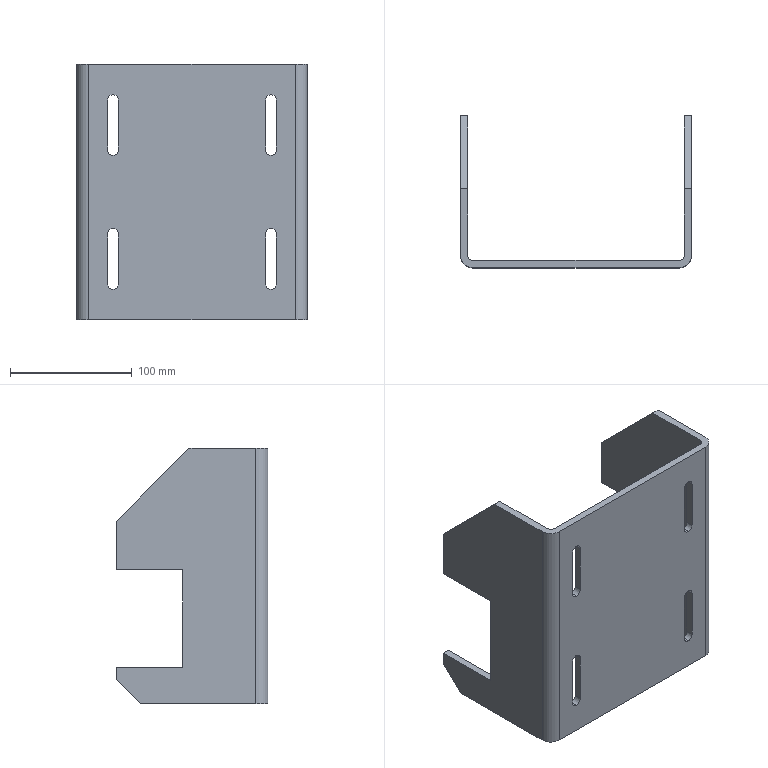Part | SolidWorks | features Chamfer 2, ICE 2, Extrusion 1 | 1 solid | 46 faces | box 190 x 125 x 210 mm | volume 444526 mm3 | plane 30 | cylinder 16 | commonest cylinder face diameters 9 x12 8 x2 20 x2
STEP:
#1=CARTESIAN_POINT('',(160.,-119.,135.));
#2=VERTEX_POINT('',#1);
#3=CARTESIAN_POINT('',(164.5,-119.,139.5));
#4=VERTEX_POINT('',#3);
#5=CARTESIAN_POINT('',(160.,-119.,139.5));
#6=DIRECTION('',(0.,-1.,0.));
#7=DIRECTION('',(0.,0.,-1.));
#8=AXIS2_PLACEMENT_3D('',#5,#6,#7);
#9=CIRCLE('',#8,4.5);
#10=EDGE_CURVE('',#2,#4,#9,.T.);
#11=ORIENTED_EDGE('',*,*,#10,.F.);
#12=CARTESIAN_POINT('',(160.,-125.,135.));
#13=VERTEX_POINT('',#12);
#14=CARTESIAN_POINT('',(160.,292.,135.));
#15=DIRECTION('',(0.,-1.,0.));
#16=VECTOR('',#15,1000.);
#17=LINE('',#14,#16);
#18=EDGE_CURVE('',#2,#13,#17,.T.);
#19=ORIENTED_EDGE('',*,*,#18,.T.);
#20=CARTESIAN_POINT('',(164.5,-125.,139.5));
#21=VERTEX_POINT('',#20);
#22=CARTESIAN_POINT('',(160.,-125.,139.5));
#23=DIRECTION('',(0.,-1.,0.));
#24=DIRECTION('',(0.,0.,-1.));
#25=AXIS2_PLACEMENT_3D('',#22,#23,#24);
#26=CIRCLE('',#25,4.5);
#27=EDGE_CURVE('',#13,#21,#26,.T.);
#28=ORIENTED_EDGE('',*,*,#27,.T.);
#29=CARTESIAN_POINT('',(164.5,292.,139.5));
#30=DIRECTION('',(0.,-1.,0.));
#31=VECTOR('',#30,1000.);
#32=LINE('',#29,#31);
#33=EDGE_CURVE('',#4,#21,#32,.T.);
#34=ORIENTED_EDGE('',*,*,#33,.F.);
#35=EDGE_LOOP('',(#11,#19,#28,#34));
#36=FACE_OUTER_BOUND('',#35,.T.);
#37=CARTESIAN_POINT('',(160.,292.,139.5));
#38=DIRECTION('',(0.,-1.,0.));
#39=DIRECTION('',(0.,0.,-1.));
#40=AXIS2_PLACEMENT_3D('',#37,#38,#39);
#41=CYLINDRICAL_SURFACE('',#40,4.5);
#42=ADVANCED_FACE('',(#36),#41,.F.);
#43=CARTESIAN_POINT('',(30.,-119.,25.));
#44=VERTEX_POINT('',#43);
#45=CARTESIAN_POINT('',(34.5,-119.,29.5));
#46=VERTEX_POINT('',#45);
#47=CARTESIAN_POINT('',(30.,-119.,29.5));
#48=DIRECTION('',(0.,-1.,0.));
#49=DIRECTION('',(0.,0.,-1.));
#50=AXIS2_PLACEMENT_3D('',#47,#48,#49);
#51=CIRCLE('',#50,4.5);
#52=EDGE_CURVE('',#44,#46,#51,.T.);
#53=ORIENTED_EDGE('',*,*,#52,.F.);
#54=CARTESIAN_POINT('',(30.,-125.,25.));
#55=VERTEX_POINT('',#54);
#56=CARTESIAN_POINT('',(30.,292.,25.));
#57=DIRECTION('',(0.,-1.,0.));
#58=VECTOR('',#57,1000.);
#59=LINE('',#56,#58);
#60=EDGE_CURVE('',#44,#55,#59,.T.);
#61=ORIENTED_EDGE('',*,*,#60,.T.);
#62=CARTESIAN_POINT('',(34.5,-125.,29.5));
#63=VERTEX_POINT('',#62);
#64=CARTESIAN_POINT('',(30.,-125.,29.5));
#65=DIRECTION('',(0.,-1.,0.));
#66=DIRECTION('',(0.,0.,-1.));
#67=AXIS2_PLACEMENT_3D('',#64,#65,#66);
#68=CIRCLE('',#67,4.5);
#69=EDGE_CURVE('',#55,#63,#68,.T.);
#70=ORIENTED_EDGE('',*,*,#69,.T.);
#71=CARTESIAN_POINT('',(34.5,292.,29.5));
#72=DIRECTION('',(0.,-1.,0.));
#73=VECTOR('',#72,1000.);
#74=LINE('',#71,#73);
#75=EDGE_CURVE('',#46,#63,#74,.T.);
#76=ORIENTED_EDGE('',*,*,#75,.F.);
#77=EDGE_LOOP('',(#53,#61,#70,#76));
#78=FACE_OUTER_BOUND('',#77,.T.);
#79=CARTESIAN_POINT('',(30.,292.,29.5));
#80=DIRECTION('',(0.,-1.,0.));
#81=DIRECTION('',(0.,0.,-1.));
#82=AXIS2_PLACEMENT_3D('',#79,#80,#81);
#83=CYLINDRICAL_SURFACE('',#82,4.5);
#84=ADVANCED_FACE('',(#78),#83,.F.);
#85=CARTESIAN_POINT('',(160.,-119.,25.));
#86=VERTEX_POINT('',#85);
#87=CARTESIAN_POINT('',(164.5,-119.,29.5));
#88=VERTEX_POINT('',#87);
#89=CARTESIAN_POINT('',(160.,-119.,29.5));
#90=DIRECTION('',(0.,-1.,0.));
#91=DIRECTION('',(0.,0.,-1.));
#92=AXIS2_PLACEMENT_3D('',#89,#90,#91);
#93=CIRCLE('',#92,4.5);
#94=EDGE_CURVE('',#86,#88,#93,.T.);
#95=ORIENTED_EDGE('',*,*,#94,.F.);
#96=CARTESIAN_POINT('',(160.,-125.,25.));
#97=VERTEX_POINT('',#96);
#98=CARTESIAN_POINT('',(160.,292.,25.));
#99=DIRECTION('',(0.,-1.,0.));
#100=VECTOR('',#99,1000.);
#101=LINE('',#98,#100);
#102=EDGE_CURVE('',#86,#97,#101,.T.);
#103=ORIENTED_EDGE('',*,*,#102,.T.);
#104=CARTESIAN_POINT('',(164.5,-125.,29.5));
#105=VERTEX_POINT('',#104);
#106=CARTESIAN_POINT('',(160.,-125.,29.5));
#107=DIRECTION('',(0.,-1.,0.));
#108=DIRECTION('',(0.,0.,-1.));
#109=AXIS2_PLACEMENT_3D('',#106,#107,#108);
#110=CIRCLE('',#109,4.5);
#111=EDGE_CURVE('',#97,#105,#110,.T.);
#112=ORIENTED_EDGE('',*,*,#111,.T.);
#113=CARTESIAN_POINT('',(164.5,292.,29.5));
#114=DIRECTION('',(0.,-1.,0.));
#115=VECTOR('',#114,1000.);
#116=LINE('',#113,#115);
#117=EDGE_CURVE('',#88,#105,#116,.T.);
#118=ORIENTED_EDGE('',*,*,#117,.F.);
#119=EDGE_LOOP('',(#95,#103,#112,#118));
#120=FACE_OUTER_BOUND('',#119,.T.);
#121=CARTESIAN_POINT('',(160.,292.,29.5));
#122=DIRECTION('',(0.,-1.,0.));
#123=DIRECTION('',(0.,0.,-1.));
#124=AXIS2_PLACEMENT_3D('',#121,#122,#123);
#125=CYLINDRICAL_SURFACE('',#124,4.5);
#126=ADVANCED_FACE('',(#120),#125,.F.);
#127=CARTESIAN_POINT('',(30.,-119.,135.));
#128=VERTEX_POINT('',#127);
#129=CARTESIAN_POINT('',(34.5,-119.,139.5));
#130=VERTEX_POINT('',#129);
#131=CARTESIAN_POINT('',(30.,-119.,139.5));
#132=DIRECTION('',(0.,-1.,0.));
#133=DIRECTION('',(0.,0.,-1.));
#134=AXIS2_PLACEMENT_3D('',#131,#132,#133);
#135=CIRCLE('',#134,4.5);
#136=EDGE_CURVE('',#128,#130,#135,.T.);
#137=ORIENTED_EDGE('',*,*,#136,.F.);
#138=CARTESIAN_POINT('',(30.,-125.,135.));
#139=VERTEX_POINT('',#138);
#140=CARTESIAN_POINT('',(30.,292.,135.));
#141=DIRECTION('',(0.,-1.,0.));
#142=VECTOR('',#141,1000.);
#143=LINE('',#140,#142);
#144=EDGE_CURVE('',#128,#139,#143,.T.);
#145=ORIENTED_EDGE('',*,*,#144,.T.);
#146=CARTESIAN_POINT('',(34.5,-125.,139.5));
#147=VERTEX_POINT('',#146);
#148=CARTESIAN_POINT('',(30.,-125.,139.5));
#149=DIRECTION('',(0.,-1.,0.));
#150=DIRECTION('',(0.,0.,-1.));
#151=AXIS2_PLACEMENT_3D('',#148,#149,#150);
#152=CIRCLE('',#151,4.5);
#153=EDGE_CURVE('',#139,#147,#152,.T.);
#154=ORIENTED_EDGE('',*,*,#153,.T.);
#155=CARTESIAN_POINT('',(34.5,292.,139.5));
#156=DIRECTION('',(0.,-1.,0.));
#157=VECTOR('',#156,1000.);
#158=LINE('',#155,#157);
#159=EDGE_CURVE('',#130,#147,#158,.T.);
#160=ORIENTED_EDGE('',*,*,#159,.F.);
#161=EDGE_LOOP('',(#137,#145,#154,#160));
#162=FACE_OUTER_BOUND('',#161,.T.);
#163=CARTESIAN_POINT('',(30.,292.,139.5));
#164=DIRECTION('',(0.,-1.,0.));
#165=DIRECTION('',(0.,0.,-1.));
#166=AXIS2_PLACEMENT_3D('',#163,#164,#165);
#167=CYLINDRICAL_SURFACE('',#166,4.5);
#168=ADVANCED_FACE('',(#162),#167,.F.);
#169=CARTESIAN_POINT('',(6.,0.,150.));
#170=VERTEX_POINT('',#169);
#171=CARTESIAN_POINT('',(6.,0.,110.));
#172=VERTEX_POINT('',#171);
#173=CARTESIAN_POINT('',(6.,0.,210.));
#174=DIRECTION('',(0.,0.,-1.));
#175=VECTOR('',#174,1000.);
#176=LINE('',#173,#175);
#177=EDGE_CURVE('',#170,#172,#176,.T.);
#178=ORIENTED_EDGE('',*,*,#177,.T.);
#179=CARTESIAN_POINT('',(0.,0.,110.));
#180=VERTEX_POINT('',#179);
#181=CARTESIAN_POINT('',(6.,0.,110.));
#182=DIRECTION('',(-1.,0.,0.));
#183=VECTOR('',#182,1000.);
#184=LINE('',#181,#183);
#185=EDGE_CURVE('',#172,#180,#184,.T.);
#186=ORIENTED_EDGE('',*,*,#185,.T.);
#187=CARTESIAN_POINT('',(0.,0.,150.));
#188=VERTEX_POINT('',#187);
#189=CARTESIAN_POINT('',(0.,0.,210.));
#190=DIRECTION('',(0.,0.,-1.));
#191=VECTOR('',#190,1000.);
#192=LINE('',#189,#191);
#193=EDGE_CURVE('',#188,#180,#192,.T.);
#194=ORIENTED_EDGE('',*,*,#193,.F.);
#195=CARTESIAN_POINT('',(6.,0.,150.));
#196=DIRECTION('',(1.,0.,0.));
#197=VECTOR('',#196,1000.);
#198=LINE('',#195,#197);
#199=EDGE_CURVE('',#188,#170,#198,.T.);
#200=ORIENTED_EDGE('',*,*,#199,.T.);
#201=EDGE_LOOP('',(#178,#186,#194,#200));
#202=FACE_OUTER_BOUND('',#201,.T.);
#203=CARTESIAN_POINT('',(6.,0.,210.));
#204=DIRECTION('',(0.,-1.,0.));
#205=DIRECTION('',(0.,0.,-1.));
#206=AXIS2_PLACEMENT_3D('',#203,#204,#205);
#207=PLANE('',#206);
#208=ADVANCED_FACE('',(#202),#207,.F.);
#209=CARTESIAN_POINT('',(190.,0.,150.));
#210=VERTEX_POINT('',#209);
#211=CARTESIAN_POINT('',(190.,0.,110.));
#212=VERTEX_POINT('',#211);
#213=CARTESIAN_POINT('',(190.,0.,210.));
#214=DIRECTION('',(0.,0.,-1.));
#215=VECTOR('',#214,1000.);
#216=LINE('',#213,#215);
#217=EDGE_CURVE('',#210,#212,#216,.T.);
#218=ORIENTED_EDGE('',*,*,#217,.T.);
#219=CARTESIAN_POINT('',(184.,0.,110.));
#220=VERTEX_POINT('',#219);
#221=CARTESIAN_POINT('',(190.,0.,110.));
#222=DIRECTION('',(-1.,0.,0.));
#223=VECTOR('',#222,1000.);
#224=LINE('',#221,#223);
#225=EDGE_CURVE('',#212,#220,#224,.T.);
#226=ORIENTED_EDGE('',*,*,#225,.T.);
#227=CARTESIAN_POINT('',(184.,0.,150.));
#228=VERTEX_POINT('',#227);
#229=CARTESIAN_POINT('',(184.,0.,210.));
#230=DIRECTION('',(0.,0.,-1.));
#231=VECTOR('',#230,1000.);
#232=LINE('',#229,#231);
#233=EDGE_CURVE('',#228,#220,#232,.T.);
#234=ORIENTED_EDGE('',*,*,#233,.F.);
#235=CARTESIAN_POINT('',(190.,0.,150.));
#236=DIRECTION('',(1.,0.,0.));
#237=VECTOR('',#236,1000.);
#238=LINE('',#235,#237);
#239=EDGE_CURVE('',#228,#210,#238,.T.);
#240=ORIENTED_EDGE('',*,*,#239,.T.);
#241=EDGE_LOOP('',(#218,#226,#234,#240));
#242=FACE_OUTER_BOUND('',#241,.T.);
#243=CARTESIAN_POINT('',(190.,0.,210.));
#244=DIRECTION('',(0.,-1.,0.));
#245=DIRECTION('',(0.,0.,-1.));
#246=AXIS2_PLACEMENT_3D('',#243,#244,#245);
#247=PLANE('',#246);
#248=ADVANCED_FACE('',(#242),#247,.F.);
#249=CARTESIAN_POINT('',(0.,0.,30.));
#250=VERTEX_POINT('',#249);
#251=CARTESIAN_POINT('',(0.,0.,20.));
#252=VERTEX_POINT('',#251);
#253=CARTESIAN_POINT('',(0.,0.,210.));
#254=DIRECTION('',(0.,0.,-1.));
#255=VECTOR('',#254,1000.);
#256=LINE('',#253,#255);
#257=EDGE_CURVE('',#250,#252,#256,.T.);
#258=ORIENTED_EDGE('',*,*,#257,.F.);
#259=CARTESIAN_POINT('',(6.,0.,30.));
#260=VERTEX_POINT('',#259);
#261=CARTESIAN_POINT('',(6.,0.,30.));
#262=DIRECTION('',(1.,0.,0.));
#263=VECTOR('',#262,1000.);
#264=LINE('',#261,#263);
#265=EDGE_CURVE('',#250,#260,#264,.T.);
#266=ORIENTED_EDGE('',*,*,#265,.T.);
#267=CARTESIAN_POINT('',(6.,0.,20.));
#268=VERTEX_POINT('',#267);
#269=CARTESIAN_POINT('',(6.,0.,210.));
#270=DIRECTION('',(0.,0.,-1.));
#271=VECTOR('',#270,1000.);
#272=LINE('',#269,#271);
#273=EDGE_CURVE('',#260,#268,#272,.T.);
#274=ORIENTED_EDGE('',*,*,#273,.T.);
#275=CARTESIAN_POINT('',(6.,0.,20.));
#276=DIRECTION('',(-1.,0.,0.));
#277=VECTOR('',#276,1000.);
#278=LINE('',#275,#277);
#279=EDGE_CURVE('',#268,#252,#278,.T.);
#280=ORIENTED_EDGE('',*,*,#279,.T.);
#281=EDGE_LOOP('',(#258,#266,#274,#280));
#282=FACE_OUTER_BOUND('',#281,.T.);
#283=CARTESIAN_POINT('',(6.,0.,210.));
#284=DIRECTION('',(0.,-1.,0.));
#285=DIRECTION('',(0.,0.,-1.));
#286=AXIS2_PLACEMENT_3D('',#283,#284,#285);
#287=PLANE('',#286);
#288=ADVANCED_FACE('',(#282),#287,.F.);
#289=ORIENTED_EDGE('',*,*,#193,.T.);
#290=CARTESIAN_POINT('',(0.,-55.,110.));
#291=VERTEX_POINT('',#290);
#292=CARTESIAN_POINT('',(0.,0.,110.));
#293=DIRECTION('',(0.,-1.,0.));
#294=VECTOR('',#293,1000.);
#295=LINE('',#292,#294);
#296=EDGE_CURVE('',#180,#291,#295,.T.);
#297=ORIENTED_EDGE('',*,*,#296,.T.);
#298=CARTESIAN_POINT('',(0.,-55.,30.));
#299=VERTEX_POINT('',#298);
#300=CARTESIAN_POINT('',(0.,-55.,210.));
#301=DIRECTION('',(0.,0.,-1.));
#302=VECTOR('',#301,1000.);
#303=LINE('',#300,#302);
#304=EDGE_CURVE('',#291,#299,#303,.T.);
#305=ORIENTED_EDGE('',*,*,#304,.T.);
#306=CARTESIAN_POINT('',(0.,0.,30.));
#307=DIRECTION('',(0.,1.,0.));
#308=VECTOR('',#307,1000.);
#309=LINE('',#306,#308);
#310=EDGE_CURVE('',#299,#250,#309,.T.);
#311=ORIENTED_EDGE('',*,*,#310,.T.);
#312=ORIENTED_EDGE('',*,*,#257,.T.);
#313=CARTESIAN_POINT('',(0.,-20.,0.));
#314=VERTEX_POINT('',#313);
#315=CARTESIAN_POINT('',(0.,0.,20.));
#316=DIRECTION('',(0.,-0.7071,-0.7071));
#317=VECTOR('',#316,1000.);
#318=LINE('',#315,#317);
#319=EDGE_CURVE('',#252,#314,#318,.T.);
#320=ORIENTED_EDGE('',*,*,#319,.T.);
#321=CARTESIAN_POINT('',(0.,-115.,0.));
#322=VERTEX_POINT('',#321);
#323=CARTESIAN_POINT('',(0.,0.,0.));
#324=DIRECTION('',(0.,-1.,0.));
#325=VECTOR('',#324,1000.);
#326=LINE('',#323,#325);
#327=EDGE_CURVE('',#314,#322,#326,.T.);
#328=ORIENTED_EDGE('',*,*,#327,.T.);
#329=CARTESIAN_POINT('',(0.,-115.,210.));
#330=VERTEX_POINT('',#329);
#331=CARTESIAN_POINT('',(0.,-115.,210.));
#332=DIRECTION('',(0.,0.,-1.));
#333=VECTOR('',#332,1000.);
#334=LINE('',#331,#333);
#335=EDGE_CURVE('',#330,#322,#334,.T.);
#336=ORIENTED_EDGE('',*,*,#335,.F.);
#337=CARTESIAN_POINT('',(0.,-60.,210.));
#338=VERTEX_POINT('',#337);
#339=CARTESIAN_POINT('',(0.,0.,210.));
#340=DIRECTION('',(0.,-1.,0.));
#341=VECTOR('',#340,1000.);
#342=LINE('',#339,#341);
#343=EDGE_CURVE('',#338,#330,#342,.T.);
#344=ORIENTED_EDGE('',*,*,#343,.F.);
#345=CARTESIAN_POINT('',(0.,-60.,210.));
#346=DIRECTION('',(0.,0.7071,-0.7071));
#347=VECTOR('',#346,1000.);
#348=LINE('',#345,#347);
#349=EDGE_CURVE('',#338,#188,#348,.T.);
#350=ORIENTED_EDGE('',*,*,#349,.T.);
#351=EDGE_LOOP('',(#289,#297,#305,#311,#312,#320,#328,#336,#344,#350));
#352=FACE_OUTER_BOUND('',#351,.T.);
#353=CARTESIAN_POINT('',(0.,0.,210.));
#354=DIRECTION('',(1.,0.,0.));
#355=DIRECTION('',(0.,0.,-1.));
#356=AXIS2_PLACEMENT_3D('',#353,#354,#355);
#357=PLANE('',#356);
#358=ADVANCED_FACE('',(#352),#357,.F.);
#359=CARTESIAN_POINT('',(10.,-125.,0.));
#360=VERTEX_POINT('',#359);
#361=CARTESIAN_POINT('',(10.,-115.,0.));
#362=DIRECTION('',(0.,0.,1.));
#363=DIRECTION('',(1.,0.,0.));
#364=AXIS2_PLACEMENT_3D('',#361,#362,#363);
#365=CIRCLE('',#364,10.);
#366=EDGE_CURVE('',#322,#360,#365,.T.);
#367=ORIENTED_EDGE('',*,*,#366,.T.);
#368=CARTESIAN_POINT('',(10.,-125.,210.));
#369=VERTEX_POINT('',#368);
#370=CARTESIAN_POINT('',(10.,-125.,210.));
#371=DIRECTION('',(0.,0.,-1.));
#372=VECTOR('',#371,1000.);
#373=LINE('',#370,#372);
#374=EDGE_CURVE('',#369,#360,#373,.T.);
#375=ORIENTED_EDGE('',*,*,#374,.F.);
#376=CARTESIAN_POINT('',(10.,-115.,210.));
#377=DIRECTION('',(0.,0.,1.));
#378=DIRECTION('',(1.,0.,0.));
#379=AXIS2_PLACEMENT_3D('',#376,#377,#378);
#380=CIRCLE('',#379,10.);
#381=EDGE_CURVE('',#330,#369,#380,.T.);
#382=ORIENTED_EDGE('',*,*,#381,.F.);
#383=ORIENTED_EDGE('',*,*,#335,.T.);
#384=EDGE_LOOP('',(#367,#375,#382,#383));
#385=FACE_OUTER_BOUND('',#384,.T.);
#386=CARTESIAN_POINT('',(10.,-115.,210.));
#387=DIRECTION('',(0.,0.,-1.));
#388=DIRECTION('',(-1.,0.,0.));
#389=AXIS2_PLACEMENT_3D('',#386,#387,#388);
#390=CYLINDRICAL_SURFACE('',#389,10.);
#391=ADVANCED_FACE('',(#385),#390,.T.);
#392=CARTESIAN_POINT('',(155.5,-125.,180.5));
#393=VERTEX_POINT('',#392);
#394=CARTESIAN_POINT('',(155.5,-125.,139.5));
#395=VERTEX_POINT('',#394);
#396=CARTESIAN_POINT('',(155.5,-125.,180.5));
#397=DIRECTION('',(0.,0.,-1.));
#398=VECTOR('',#397,1000.);
#399=LINE('',#396,#398);
#400=EDGE_CURVE('',#393,#395,#399,.T.);
#401=ORIENTED_EDGE('',*,*,#400,.F.);
#402=CARTESIAN_POINT('',(164.5,-125.,180.5));
#403=VERTEX_POINT('',#402);
#404=CARTESIAN_POINT('',(160.,-125.,180.5));
#405=DIRECTION('',(0.,-1.,0.));
#406=DIRECTION('',(0.,0.,-1.));
#407=AXIS2_PLACEMENT_3D('',#404,#405,#406);
#408=CIRCLE('',#407,4.5);
#409=EDGE_CURVE('',#403,#393,#408,.T.);
#410=ORIENTED_EDGE('',*,*,#409,.F.);
#411=CARTESIAN_POINT('',(164.5,-125.,180.5));
#412=DIRECTION('',(0.,0.,1.));
#413=VECTOR('',#412,1000.);
#414=LINE('',#411,#413);
#415=EDGE_CURVE('',#21,#403,#414,.T.);
#416=ORIENTED_EDGE('',*,*,#415,.F.);
#417=ORIENTED_EDGE('',*,*,#27,.F.);
#418=CARTESIAN_POINT('',(160.,-125.,139.5));
#419=DIRECTION('',(0.,-1.,0.));
#420=DIRECTION('',(0.,0.,-1.));
#421=AXIS2_PLACEMENT_3D('',#418,#419,#420);
#422=CIRCLE('',#421,4.5);
#423=EDGE_CURVE('',#395,#13,#422,.T.);
#424=ORIENTED_EDGE('',*,*,#423,.F.);
#425=EDGE_LOOP('',(#401,#410,#416,#417,#424));
#426=FACE_BOUND('',#425,.T.);
#427=CARTESIAN_POINT('',(25.5,-125.,70.5));
#428=VERTEX_POINT('',#427);
#429=CARTESIAN_POINT('',(25.5,-125.,29.5));
#430=VERTEX_POINT('',#429);
#431=CARTESIAN_POINT('',(25.5,-125.,70.5));
#432=DIRECTION('',(0.,0.,-1.));
#433=VECTOR('',#432,1000.);
#434=LINE('',#431,#433);
#435=EDGE_CURVE('',#428,#430,#434,.T.);
#436=ORIENTED_EDGE('',*,*,#435,.F.);
#437=CARTESIAN_POINT('',(34.5,-125.,70.5));
#438=VERTEX_POINT('',#437);
#439=CARTESIAN_POINT('',(30.,-125.,70.5));
#440=DIRECTION('',(0.,-1.,0.));
#441=DIRECTION('',(0.,0.,-1.));
#442=AXIS2_PLACEMENT_3D('',#439,#440,#441);
#443=CIRCLE('',#442,4.5);
#444=EDGE_CURVE('',#438,#428,#443,.T.);
#445=ORIENTED_EDGE('',*,*,#444,.F.);
#446=CARTESIAN_POINT('',(34.5,-125.,70.5));
#447=DIRECTION('',(0.,0.,1.));
#448=VECTOR('',#447,1000.);
#449=LINE('',#446,#448);
#450=EDGE_CURVE('',#63,#438,#449,.T.);
#451=ORIENTED_EDGE('',*,*,#450,.F.);
#452=ORIENTED_EDGE('',*,*,#69,.F.);
#453=CARTESIAN_POINT('',(30.,-125.,29.5));
#454=DIRECTION('',(0.,-1.,0.));
#455=DIRECTION('',(0.,0.,-1.));
#456=AXIS2_PLACEMENT_3D('',#453,#454,#455);
#457=CIRCLE('',#456,4.5);
#458=EDGE_CURVE('',#430,#55,#457,.T.);
#459=ORIENTED_EDGE('',*,*,#458,.F.);
#460=EDGE_LOOP('',(#436,#445,#451,#452,#459));
#461=FACE_BOUND('',#460,.T.);
#462=CARTESIAN_POINT('',(155.5,-125.,70.5));
#463=VERTEX_POINT('',#462);
#464=CARTESIAN_POINT('',(155.5,-125.,29.5));
#465=VERTEX_POINT('',#464);
#466=CARTESIAN_POINT('',(155.5,-125.,70.5));
#467=DIRECTION('',(0.,0.,-1.));
#468=VECTOR('',#467,1000.);
#469=LINE('',#466,#468);
#470=EDGE_CURVE('',#463,#465,#469,.T.);
#471=ORIENTED_EDGE('',*,*,#470,.F.);
#472=CARTESIAN_POINT('',(164.5,-125.,70.5));
#473=VERTEX_POINT('',#472);
#474=CARTESIAN_POINT('',(160.,-125.,70.5));
#475=DIRECTION('',(0.,-1.,0.));
#476=DIRECTION('',(0.,0.,-1.));
#477=AXIS2_PLACEMENT_3D('',#474,#475,#476);
#478=CIRCLE('',#477,4.5);
#479=EDGE_CURVE('',#473,#463,#478,.T.);
#480=ORIENTED_EDGE('',*,*,#479,.F.);
#481=CARTESIAN_POINT('',(164.5,-125.,70.5));
#482=DIRECTION('',(0.,0.,1.));
#483=VECTOR('',#482,1000.);
#484=LINE('',#481,#483);
#485=EDGE_CURVE('',#105,#473,#484,.T.);
#486=ORIENTED_EDGE('',*,*,#485,.F.);
#487=ORIENTED_EDGE('',*,*,#111,.F.);
#488=CARTESIAN_POINT('',(160.,-125.,29.5));
#489=DIRECTION('',(0.,-1.,0.));
#490=DIRECTION('',(0.,0.,-1.));
#491=AXIS2_PLACEMENT_3D('',#488,#489,#490);
#492=CIRCLE('',#491,4.5);
#493=EDGE_CURVE('',#465,#97,#492,.T.);
#494=ORIENTED_EDGE('',*,*,#493,.F.);
#495=EDGE_LOOP('',(#471,#480,#486,#487,#494));
#496=FACE_BOUND('',#495,.T.);
#497=CARTESIAN_POINT('',(25.5,-125.,180.5));
#498=VERTEX_POINT('',#497);
#499=CARTESIAN_POINT('',(25.5,-125.,139.5));
#500=VERTEX_POINT('',#499);
#501=CARTESIAN_POINT('',(25.5,-125.,180.5));
#502=DIRECTION('',(0.,0.,-1.));
#503=VECTOR('',#502,1000.);
#504=LINE('',#501,#503);
#505=EDGE_CURVE('',#498,#500,#504,.T.);
#506=ORIENTED_EDGE('',*,*,#505,.F.);
#507=CARTESIAN_POINT('',(34.5,-125.,180.5));
#508=VERTEX_POINT('',#507);
#509=CARTESIAN_POINT('',(30.,-125.,180.5));
#510=DIRECTION('',(0.,-1.,0.));
#511=DIRECTION('',(0.,0.,-1.));
#512=AXIS2_PLACEMENT_3D('',#509,#510,#511);
#513=CIRCLE('',#512,4.5);
#514=EDGE_CURVE('',#508,#498,#513,.T.);
#515=ORIENTED_EDGE('',*,*,#514,.F.);
#516=CARTESIAN_POINT('',(34.5,-125.,180.5));
#517=DIRECTION('',(0.,0.,1.));
#518=VECTOR('',#517,1000.);
#519=LINE('',#516,#518);
#520=EDGE_CURVE('',#147,#508,#519,.T.);
#521=ORIENTED_EDGE('',*,*,#520,.F.);
#522=ORIENTED_EDGE('',*,*,#153,.F.);
#523=CARTESIAN_POINT('',(30.,-125.,139.5));
#524=DIRECTION('',(0.,-1.,0.));
#525=DIRECTION('',(0.,0.,-1.));
#526=AXIS2_PLACEMENT_3D('',#523,#524,#525);
#527=CIRCLE('',#526,4.5);
#528=EDGE_CURVE('',#500,#139,#527,.T.);
#529=ORIENTED_EDGE('',*,*,#528,.F.);
#530=EDGE_LOOP('',(#506,#515,#521,#522,#529));
#531=FACE_BOUND('',#530,.T.);
#532=CARTESIAN_POINT('',(180.,-125.,0.));
#533=VERTEX_POINT('',#532);
#534=CARTESIAN_POINT('',(10.,-125.,0.));
#535=DIRECTION('',(1.,0.,0.));
#536=VECTOR('',#535,1000.);
#537=LINE('',#534,#536);
#538=EDGE_CURVE('',#360,#533,#537,.T.);
#539=ORIENTED_EDGE('',*,*,#538,.T.);
#540=CARTESIAN_POINT('',(180.,-125.,210.));
#541=VERTEX_POINT('',#540);
#542=CARTESIAN_POINT('',(180.,-125.,210.));
#543=DIRECTION('',(0.,0.,-1.));
#544=VECTOR('',#543,1000.);
#545=LINE('',#542,#544);
#546=EDGE_CURVE('',#541,#533,#545,.T.);
#547=ORIENTED_EDGE('',*,*,#546,.F.);
#548=CARTESIAN_POINT('',(10.,-125.,210.));
#549=DIRECTION('',(1.,0.,0.));
#550=VECTOR('',#549,1000.);
#551=LINE('',#548,#550);
#552=EDGE_CURVE('',#369,#541,#551,.T.);
#553=ORIENTED_EDGE('',*,*,#552,.F.);
#554=ORIENTED_EDGE('',*,*,#374,.T.);
#555=EDGE_LOOP('',(#539,#547,#553,#554));
#556=FACE_OUTER_BOUND('',#555,.T.);
#557=CARTESIAN_POINT('',(10.,-125.,210.));
#558=DIRECTION('',(0.,1.,0.));
#559=DIRECTION('',(0.,0.,1.));
#560=AXIS2_PLACEMENT_3D('',#557,#558,#559);
#561=PLANE('',#560);
#562=ADVANCED_FACE('',(#426,#461,#496,#531,#556),#561,.F.);
#563=CARTESIAN_POINT('',(190.,-115.,0.));
#564=VERTEX_POINT('',#563);
#565=CARTESIAN_POINT('',(180.,-115.,0.));
#566=DIRECTION('',(0.,0.,1.));
#567=DIRECTION('',(1.,0.,0.));
#568=AXIS2_PLACEMENT_3D('',#565,#566,#567);
#569=CIRCLE('',#568,10.);
#570=EDGE_CURVE('',#533,#564,#569,.T.);
#571=ORIENTED_EDGE('',*,*,#570,.T.);
#572=CARTESIAN_POINT('',(190.,-115.,210.));
#573=VERTEX_POINT('',#572);
#574=CARTESIAN_POINT('',(190.,-115.,210.));
#575=DIRECTION('',(0.,0.,-1.));
#576=VECTOR('',#575,1000.);
#577=LINE('',#574,#576);
#578=EDGE_CURVE('',#573,#564,#577,.T.);
#579=ORIENTED_EDGE('',*,*,#578,.F.);
#580=CARTESIAN_POINT('',(180.,-115.,210.));
#581=DIRECTION('',(0.,0.,1.));
#582=DIRECTION('',(1.,0.,0.));
#583=AXIS2_PLACEMENT_3D('',#580,#581,#582);
#584=CIRCLE('',#583,10.);
#585=EDGE_CURVE('',#541,#573,#584,.T.);
#586=ORIENTED_EDGE('',*,*,#585,.F.);
#587=ORIENTED_EDGE('',*,*,#546,.T.);
#588=EDGE_LOOP('',(#571,#579,#586,#587));
#589=FACE_OUTER_BOUND('',#588,.T.);
#590=CARTESIAN_POINT('',(180.,-115.,210.));
#591=DIRECTION('',(0.,0.,-1.));
#592=DIRECTION('',(-1.,0.,0.));
#593=AXIS2_PLACEMENT_3D('',#590,#591,#592);
#594=CYLINDRICAL_SURFACE('',#593,10.);
#595=ADVANCED_FACE('',(#589),#594,.T.);
#596=CARTESIAN_POINT('',(190.,-55.,110.));
#597=VERTEX_POINT('',#596);
#598=CARTESIAN_POINT('',(190.,-55.,30.));
#599=VERTEX_POINT('',#598);
#600=CARTESIAN_POINT('',(190.,-55.,30.));
#601=DIRECTION('',(0.,0.,-1.));
#602=VECTOR('',#601,1000.);
#603=LINE('',#600,#602);
#604=EDGE_CURVE('',#597,#599,#603,.T.);
#605=ORIENTED_EDGE('',*,*,#604,.F.);
#606=CARTESIAN_POINT('',(190.,-55.,110.));
#607=DIRECTION('',(0.,-1.,0.));
#608=VECTOR('',#607,1000.);
#609=LINE('',#606,#608);
#610=EDGE_CURVE('',#212,#597,#609,.T.);
#611=ORIENTED_EDGE('',*,*,#610,.F.);
#612=ORIENTED_EDGE('',*,*,#217,.F.);
#613=CARTESIAN_POINT('',(190.,-60.,210.));
#614=VERTEX_POINT('',#613);
#615=CARTESIAN_POINT('',(190.,-60.,210.));
#616=DIRECTION('',(0.,-0.7071,0.7071));
#617=VECTOR('',#616,1000.);
#618=LINE('',#615,#617);
#619=EDGE_CURVE('',#210,#614,#618,.T.);
#620=ORIENTED_EDGE('',*,*,#619,.T.);
#621=CARTESIAN_POINT('',(190.,-115.,210.));
#622=DIRECTION('',(0.,1.,0.));
#623=VECTOR('',#622,1000.);
#624=LINE('',#621,#623);
#625=EDGE_CURVE('',#573,#614,#624,.T.);
#626=ORIENTED_EDGE('',*,*,#625,.F.);
#627=ORIENTED_EDGE('',*,*,#578,.T.);
#628=CARTESIAN_POINT('',(190.,-20.,0.));
#629=VERTEX_POINT('',#628);
#630=CARTESIAN_POINT('',(190.,-115.,0.));
#631=DIRECTION('',(0.,1.,0.));
#632=VECTOR('',#631,1000.);
#633=LINE('',#630,#632);
#634=EDGE_CURVE('',#564,#629,#633,.T.);
#635=ORIENTED_EDGE('',*,*,#634,.T.);
#636=CARTESIAN_POINT('',(190.,0.,20.));
#637=VERTEX_POINT('',#636);
#638=CARTESIAN_POINT('',(190.,0.,20.));
#639=DIRECTION('',(0.,0.7071,0.7071));
#640=VECTOR('',#639,1000.);
#641=LINE('',#638,#640);
#642=EDGE_CURVE('',#629,#637,#641,.T.);
#643=ORIENTED_EDGE('',*,*,#642,.T.);
#644=CARTESIAN_POINT('',(190.,0.,30.));
#645=VERTEX_POINT('',#644);
#646=CARTESIAN_POINT('',(190.,0.,210.));
#647=DIRECTION('',(0.,0.,-1.));
#648=VECTOR('',#647,1000.);
#649=LINE('',#646,#648);
#650=EDGE_CURVE('',#645,#637,#649,.T.);
#651=ORIENTED_EDGE('',*,*,#650,.F.);
#652=CARTESIAN_POINT('',(190.,-55.,30.));
#653=DIRECTION('',(0.,1.,0.));
#654=VECTOR('',#653,1000.);
#655=LINE('',#652,#654);
#656=EDGE_CURVE('',#599,#645,#655,.T.);
#657=ORIENTED_EDGE('',*,*,#656,.F.);
#658=EDGE_LOOP('',(#605,#611,#612,#620,#626,#627,#635,#643,#651,#657));
#659=FACE_OUTER_BOUND('',#658,.T.);
#660=CARTESIAN_POINT('',(190.,-115.,210.));
#661=DIRECTION('',(-1.,0.,0.));
#662=DIRECTION('',(0.,-1.,0.));
#663=AXIS2_PLACEMENT_3D('',#660,#661,#662);
#664=PLANE('',#663);
#665=ADVANCED_FACE('',(#659),#664,.F.);
#666=CARTESIAN_POINT('',(184.,0.,30.));
#667=VERTEX_POINT('',#666);
#668=CARTESIAN_POINT('',(184.,0.,20.));
#669=VERTEX_POINT('',#668);
#670=CARTESIAN_POINT('',(184.,0.,210.));
#671=DIRECTION('',(0.,0.,-1.));
#672=VECTOR('',#671,1000.);
#673=LINE('',#670,#672);
#674=EDGE_CURVE('',#667,#669,#673,.T.);
#675=ORIENTED_EDGE('',*,*,#674,.F.);
#676=CARTESIAN_POINT('',(190.,0.,30.));
#677=DIRECTION('',(1.,0.,0.));
#678=VECTOR('',#677,1000.);
#679=LINE('',#676,#678);
#680=EDGE_CURVE('',#667,#645,#679,.T.);
#681=ORIENTED_EDGE('',*,*,#680,.T.);
#682=ORIENTED_EDGE('',*,*,#650,.T.);
#683=CARTESIAN_POINT('',(190.,0.,20.));
#684=DIRECTION('',(-1.,0.,0.));
#685=VECTOR('',#684,1000.);
#686=LINE('',#683,#685);
#687=EDGE_CURVE('',#637,#669,#686,.T.);
#688=ORIENTED_EDGE('',*,*,#687,.T.);
#689=EDGE_LOOP('',(#675,#681,#682,#688));
#690=FACE_OUTER_BOUND('',#689,.T.);
#691=CARTESIAN_POINT('',(190.,0.,210.));
#692=DIRECTION('',(0.,-1.,0.));
#693=DIRECTION('',(0.,0.,-1.));
#694=AXIS2_PLACEMENT_3D('',#691,#692,#693);
#695=PLANE('',#694);
#696=ADVANCED_FACE('',(#690),#695,.F.);
#697=ORIENTED_EDGE('',*,*,#233,.T.);
#698=CARTESIAN_POINT('',(184.,-55.,110.));
#699=VERTEX_POINT('',#698);
#700=CARTESIAN_POINT('',(184.,-115.,110.));
#701=DIRECTION('',(0.,-1.,0.));
#702=VECTOR('',#701,1000.);
#703=LINE('',#700,#702);
#704=EDGE_CURVE('',#220,#699,#703,.T.);
#705=ORIENTED_EDGE('',*,*,#704,.T.);
#706=CARTESIAN_POINT('',(184.,-55.,30.));
#707=VERTEX_POINT('',#706);
#708=CARTESIAN_POINT('',(184.,-55.,210.));
#709=DIRECTION('',(0.,0.,-1.));
#710=VECTOR('',#709,1000.);
#711=LINE('',#708,#710);
#712=EDGE_CURVE('',#699,#707,#711,.T.);
#713=ORIENTED_EDGE('',*,*,#712,.T.);
#714=CARTESIAN_POINT('',(184.,-115.,30.));
#715=DIRECTION('',(0.,1.,0.));
#716=VECTOR('',#715,1000.);
#717=LINE('',#714,#716);
#718=EDGE_CURVE('',#707,#667,#717,.T.);
#719=ORIENTED_EDGE('',*,*,#718,.T.);
#720=ORIENTED_EDGE('',*,*,#674,.T.);
#721=CARTESIAN_POINT('',(184.,-20.,0.));
#722=VERTEX_POINT('',#721);
#723=CARTESIAN_POINT('',(184.,0.,20.));
#724=DIRECTION('',(0.,-0.7071,-0.7071));
#725=VECTOR('',#724,1000.);
#726=LINE('',#723,#725);
#727=EDGE_CURVE('',#669,#722,#726,.T.);
#728=ORIENTED_EDGE('',*,*,#727,.T.);
#729=CARTESIAN_POINT('',(184.,-115.,0.));
#730=VERTEX_POINT('',#729);
#731=CARTESIAN_POINT('',(184.,-115.,0.));
#732=DIRECTION('',(0.,-1.,0.));
#733=VECTOR('',#732,1000.);
#734=LINE('',#731,#733);
#735=EDGE_CURVE('',#722,#730,#734,.T.);
#736=ORIENTED_EDGE('',*,*,#735,.T.);
#737=CARTESIAN_POINT('',(184.,-115.,210.));
#738=VERTEX_POINT('',#737);
#739=CARTESIAN_POINT('',(184.,-115.,210.));
#740=DIRECTION('',(0.,0.,-1.));
#741=VECTOR('',#740,1000.);
#742=LINE('',#739,#741);
#743=EDGE_CURVE('',#738,#730,#742,.T.);
#744=ORIENTED_EDGE('',*,*,#743,.F.);
#745=CARTESIAN_POINT('',(184.,-60.,210.));
#746=VERTEX_POINT('',#745);
#747=CARTESIAN_POINT('',(184.,-115.,210.));
#748=DIRECTION('',(0.,-1.,0.));
#749=VECTOR('',#748,1000.);
#750=LINE('',#747,#749);
#751=EDGE_CURVE('',#746,#738,#750,.T.);
#752=ORIENTED_EDGE('',*,*,#751,.F.);
#753=CARTESIAN_POINT('',(184.,-60.,210.));
#754=DIRECTION('',(0.,0.7071,-0.7071));
#755=VECTOR('',#754,1000.);
#756=LINE('',#753,#755);
#757=EDGE_CURVE('',#746,#228,#756,.T.);
#758=ORIENTED_EDGE('',*,*,#757,.T.);
#759=EDGE_LOOP('',(#697,#705,#713,#719,#720,#728,#736,#744,#752,#758));
#760=FACE_OUTER_BOUND('',#759,.T.);
#761=CARTESIAN_POINT('',(184.,-115.,210.));
#762=DIRECTION('',(1.,0.,0.));
#763=DIRECTION('',(0.,0.,-1.));
#764=AXIS2_PLACEMENT_3D('',#761,#762,#763);
#765=PLANE('',#764);
#766=ADVANCED_FACE('',(#760),#765,.F.);
#767=CARTESIAN_POINT('',(180.,-119.,0.));
#768=VERTEX_POINT('',#767);
#769=CARTESIAN_POINT('',(180.,-115.,0.));
#770=DIRECTION('',(0.,0.,-1.));
#771=DIRECTION('',(1.,0.,0.));
#772=AXIS2_PLACEMENT_3D('',#769,#770,#771);
#773=CIRCLE('',#772,4.);
#774=EDGE_CURVE('',#730,#768,#773,.T.);
#775=ORIENTED_EDGE('',*,*,#774,.T.);
#776=CARTESIAN_POINT('',(180.,-119.,210.));
#777=VERTEX_POINT('',#776);
#778=CARTESIAN_POINT('',(180.,-119.,210.));
#779=DIRECTION('',(0.,0.,-1.));
#780=VECTOR('',#779,1000.);
#781=LINE('',#778,#780);
#782=EDGE_CURVE('',#777,#768,#781,.T.);
#783=ORIENTED_EDGE('',*,*,#782,.F.);
#784=CARTESIAN_POINT('',(180.,-115.,210.));
#785=DIRECTION('',(0.,0.,-1.));
#786=DIRECTION('',(1.,0.,0.));
#787=AXIS2_PLACEMENT_3D('',#784,#785,#786);
#788=CIRCLE('',#787,4.);
#789=EDGE_CURVE('',#738,#777,#788,.T.);
#790=ORIENTED_EDGE('',*,*,#789,.F.);
#791=ORIENTED_EDGE('',*,*,#743,.T.);
#792=EDGE_LOOP('',(#775,#783,#790,#791));
#793=FACE_OUTER_BOUND('',#792,.T.);
#794=CARTESIAN_POINT('',(180.,-115.,210.));
#795=DIRECTION('',(0.,0.,-1.));
#796=DIRECTION('',(-1.,0.,0.));
#797=AXIS2_PLACEMENT_3D('',#794,#795,#796);
#798=CYLINDRICAL_SURFACE('',#797,4.);
#799=ADVANCED_FACE('',(#793),#798,.F.);
#800=CARTESIAN_POINT('',(164.5,-119.,180.5));
#801=VERTEX_POINT('',#800);
#802=CARTESIAN_POINT('',(164.5,-119.,210.));
#803=DIRECTION('',(0.,0.,1.));
#804=VECTOR('',#803,1000.);
#805=LINE('',#802,#804);
#806=EDGE_CURVE('',#4,#801,#805,.T.);
#807=ORIENTED_EDGE('',*,*,#806,.T.);
#808=CARTESIAN_POINT('',(155.5,-119.,180.5));
#809=VERTEX_POINT('',#808);
#810=CARTESIAN_POINT('',(160.,-119.,180.5));
#811=DIRECTION('',(0.,-1.,0.));
#812=DIRECTION('',(0.,0.,-1.));
#813=AXIS2_PLACEMENT_3D('',#810,#811,#812);
#814=CIRCLE('',#813,4.5);
#815=EDGE_CURVE('',#801,#809,#814,.T.);
#816=ORIENTED_EDGE('',*,*,#815,.T.);
#817=CARTESIAN_POINT('',(155.5,-119.,139.5));
#818=VERTEX_POINT('',#817);
#819=CARTESIAN_POINT('',(155.5,-119.,210.));
#820=DIRECTION('',(0.,0.,-1.));
#821=VECTOR('',#820,1000.);
#822=LINE('',#819,#821);
#823=EDGE_CURVE('',#809,#818,#822,.T.);
#824=ORIENTED_EDGE('',*,*,#823,.T.);
#825=CARTESIAN_POINT('',(160.,-119.,139.5));
#826=DIRECTION('',(0.,-1.,0.));
#827=DIRECTION('',(0.,0.,-1.));
#828=AXIS2_PLACEMENT_3D('',#825,#826,#827);
#829=CIRCLE('',#828,4.5);
#830=EDGE_CURVE('',#818,#2,#829,.T.);
#831=ORIENTED_EDGE('',*,*,#830,.T.);
#832=ORIENTED_EDGE('',*,*,#10,.T.);
#833=EDGE_LOOP('',(#807,#816,#824,#831,#832));
#834=FACE_BOUND('',#833,.T.);
#835=CARTESIAN_POINT('',(34.5,-119.,70.5));
#836=VERTEX_POINT('',#835);
#837=CARTESIAN_POINT('',(34.5,-119.,210.));
#838=DIRECTION('',(0.,0.,1.));
#839=VECTOR('',#838,1000.);
#840=LINE('',#837,#839);
#841=EDGE_CURVE('',#46,#836,#840,.T.);
#842=ORIENTED_EDGE('',*,*,#841,.T.);
#843=CARTESIAN_POINT('',(25.5,-119.,70.5));
#844=VERTEX_POINT('',#843);
#845=CARTESIAN_POINT('',(30.,-119.,70.5));
#846=DIRECTION('',(0.,-1.,0.));
#847=DIRECTION('',(0.,0.,-1.));
#848=AXIS2_PLACEMENT_3D('',#845,#846,#847);
#849=CIRCLE('',#848,4.5);
#850=EDGE_CURVE('',#836,#844,#849,.T.);
#851=ORIENTED_EDGE('',*,*,#850,.T.);
#852=CARTESIAN_POINT('',(25.5,-119.,29.5));
#853=VERTEX_POINT('',#852);
#854=CARTESIAN_POINT('',(25.5,-119.,210.));
#855=DIRECTION('',(0.,0.,-1.));
#856=VECTOR('',#855,1000.);
#857=LINE('',#854,#856);
#858=EDGE_CURVE('',#844,#853,#857,.T.);
#859=ORIENTED_EDGE('',*,*,#858,.T.);
#860=CARTESIAN_POINT('',(30.,-119.,29.5));
#861=DIRECTION('',(0.,-1.,0.));
#862=DIRECTION('',(0.,0.,-1.));
#863=AXIS2_PLACEMENT_3D('',#860,#861,#862);
#864=CIRCLE('',#863,4.5);
#865=EDGE_CURVE('',#853,#44,#864,.T.);
#866=ORIENTED_EDGE('',*,*,#865,.T.);
#867=ORIENTED_EDGE('',*,*,#52,.T.);
#868=EDGE_LOOP('',(#842,#851,#859,#866,#867));
#869=FACE_BOUND('',#868,.T.);
#870=CARTESIAN_POINT('',(164.5,-119.,70.5));
#871=VERTEX_POINT('',#870);
#872=CARTESIAN_POINT('',(164.5,-119.,210.));
#873=DIRECTION('',(0.,0.,1.));
#874=VECTOR('',#873,1000.);
#875=LINE('',#872,#874);
#876=EDGE_CURVE('',#88,#871,#875,.T.);
#877=ORIENTED_EDGE('',*,*,#876,.T.);
#878=CARTESIAN_POINT('',(155.5,-119.,70.5));
#879=VERTEX_POINT('',#878);
#880=CARTESIAN_POINT('',(160.,-119.,70.5));
#881=DIRECTION('',(0.,-1.,0.));
#882=DIRECTION('',(0.,0.,-1.));
#883=AXIS2_PLACEMENT_3D('',#880,#881,#882);
#884=CIRCLE('',#883,4.5);
#885=EDGE_CURVE('',#871,#879,#884,.T.);
#886=ORIENTED_EDGE('',*,*,#885,.T.);
#887=CARTESIAN_POINT('',(155.5,-119.,29.5));
#888=VERTEX_POINT('',#887);
#889=CARTESIAN_POINT('',(155.5,-119.,210.));
#890=DIRECTION('',(0.,0.,-1.));
#891=VECTOR('',#890,1000.);
#892=LINE('',#889,#891);
#893=EDGE_CURVE('',#879,#888,#892,.T.);
#894=ORIENTED_EDGE('',*,*,#893,.T.);
#895=CARTESIAN_POINT('',(160.,-119.,29.5));
#896=DIRECTION('',(0.,-1.,0.));
#897=DIRECTION('',(0.,0.,-1.));
#898=AXIS2_PLACEMENT_3D('',#895,#896,#897);
#899=CIRCLE('',#898,4.5);
#900=EDGE_CURVE('',#888,#86,#899,.T.);
#901=ORIENTED_EDGE('',*,*,#900,.T.);
#902=ORIENTED_EDGE('',*,*,#94,.T.);
#903=EDGE_LOOP('',(#877,#886,#894,#901,#902));
#904=FACE_BOUND('',#903,.T.);
#905=CARTESIAN_POINT('',(34.5,-119.,180.5));
#906=VERTEX_POINT('',#905);
#907=CARTESIAN_POINT('',(34.5,-119.,210.));
#908=DIRECTION('',(0.,0.,1.));
#909=VECTOR('',#908,1000.);
#910=LINE('',#907,#909);
#911=EDGE_CURVE('',#130,#906,#910,.T.);
#912=ORIENTED_EDGE('',*,*,#911,.T.);
#913=CARTESIAN_POINT('',(25.5,-119.,180.5));
#914=VERTEX_POINT('',#913);
#915=CARTESIAN_POINT('',(30.,-119.,180.5));
#916=DIRECTION('',(0.,-1.,0.));
#917=DIRECTION('',(0.,0.,-1.));
#918=AXIS2_PLACEMENT_3D('',#915,#916,#917);
#919=CIRCLE('',#918,4.5);
#920=EDGE_CURVE('',#906,#914,#919,.T.);
#921=ORIENTED_EDGE('',*,*,#920,.T.);
#922=CARTESIAN_POINT('',(25.5,-119.,139.5));
#923=VERTEX_POINT('',#922);
#924=CARTESIAN_POINT('',(25.5,-119.,210.));
#925=DIRECTION('',(0.,0.,-1.));
#926=VECTOR('',#925,1000.);
#927=LINE('',#924,#926);
#928=EDGE_CURVE('',#914,#923,#927,.T.);
#929=ORIENTED_EDGE('',*,*,#928,.T.);
#930=CARTESIAN_POINT('',(30.,-119.,139.5));
#931=DIRECTION('',(0.,-1.,0.));
#932=DIRECTION('',(0.,0.,-1.));
#933=AXIS2_PLACEMENT_3D('',#930,#931,#932);
#934=CIRCLE('',#933,4.5);
#935=EDGE_CURVE('',#923,#128,#934,.T.);
#936=ORIENTED_EDGE('',*,*,#935,.T.);
#937=ORIENTED_EDGE('',*,*,#136,.T.);
#938=EDGE_LOOP('',(#912,#921,#929,#936,#937));
#939=FACE_BOUND('',#938,.T.);
#940=CARTESIAN_POINT('',(10.,-119.,0.));
#941=VERTEX_POINT('',#940);
#942=CARTESIAN_POINT('',(10.,-119.,0.));
#943=DIRECTION('',(-1.,0.,0.));
#944=VECTOR('',#943,1000.);
#945=LINE('',#942,#944);
#946=EDGE_CURVE('',#768,#941,#945,.T.);
#947=ORIENTED_EDGE('',*,*,#946,.T.);
#948=CARTESIAN_POINT('',(10.,-119.,210.));
#949=VERTEX_POINT('',#948);
#950=CARTESIAN_POINT('',(10.,-119.,210.));
#951=DIRECTION('',(0.,0.,-1.));
#952=VECTOR('',#951,1000.);
#953=LINE('',#950,#952);
#954=EDGE_CURVE('',#949,#941,#953,.T.);
#955=ORIENTED_EDGE('',*,*,#954,.F.);
#956=CARTESIAN_POINT('',(10.,-119.,210.));
#957=DIRECTION('',(-1.,0.,0.));
#958=VECTOR('',#957,1000.);
#959=LINE('',#956,#958);
#960=EDGE_CURVE('',#777,#949,#959,.T.);
#961=ORIENTED_EDGE('',*,*,#960,.F.);
#962=ORIENTED_EDGE('',*,*,#782,.T.);
#963=EDGE_LOOP('',(#947,#955,#961,#962));
#964=FACE_OUTER_BOUND('',#963,.T.);
#965=CARTESIAN_POINT('',(10.,-119.,210.));
#966=DIRECTION('',(0.,-1.,0.));
#967=DIRECTION('',(0.,0.,-1.));
#968=AXIS2_PLACEMENT_3D('',#965,#966,#967);
#969=PLANE('',#968);
#970=ADVANCED_FACE('',(#834,#869,#904,#939,#964),#969,.F.);
#971=CARTESIAN_POINT('',(6.,-115.,0.));
#972=VERTEX_POINT('',#971);
#973=CARTESIAN_POINT('',(10.,-115.,0.));
#974=DIRECTION('',(0.,0.,-1.));
#975=DIRECTION('',(1.,0.,0.));
#976=AXIS2_PLACEMENT_3D('',#973,#974,#975);
#977=CIRCLE('',#976,4.);
#978=EDGE_CURVE('',#941,#972,#977,.T.);
#979=ORIENTED_EDGE('',*,*,#978,.T.);
#980=CARTESIAN_POINT('',(6.,-115.,210.));
#981=VERTEX_POINT('',#980);
#982=CARTESIAN_POINT('',(6.,-115.,210.));
#983=DIRECTION('',(0.,0.,-1.));
#984=VECTOR('',#983,1000.);
#985=LINE('',#982,#984);
#986=EDGE_CURVE('',#981,#972,#985,.T.);
#987=ORIENTED_EDGE('',*,*,#986,.F.);
#988=CARTESIAN_POINT('',(10.,-115.,210.));
#989=DIRECTION('',(0.,0.,-1.));
#990=DIRECTION('',(1.,0.,0.));
#991=AXIS2_PLACEMENT_3D('',#988,#989,#990);
#992=CIRCLE('',#991,4.);
#993=EDGE_CURVE('',#949,#981,#992,.T.);
#994=ORIENTED_EDGE('',*,*,#993,.F.);
#995=ORIENTED_EDGE('',*,*,#954,.T.);
#996=EDGE_LOOP('',(#979,#987,#994,#995));
#997=FACE_OUTER_BOUND('',#996,.T.);
#998=CARTESIAN_POINT('',(10.,-115.,210.));
#999=DIRECTION('',(0.,0.,-1.));
#1000=DIRECTION('',(-1.,0.,0.));
#1001=AXIS2_PLACEMENT_3D('',#998,#999,#1000);
#1002=CYLINDRICAL_SURFACE('',#1001,4.);
#1003=ADVANCED_FACE('',(#997),#1002,.F.);
#1004=CARTESIAN_POINT('',(6.,-55.,30.));
#1005=VERTEX_POINT('',#1004);
#1006=CARTESIAN_POINT('',(6.,-55.,110.));
#1007=VERTEX_POINT('',#1006);
#1008=CARTESIAN_POINT('',(6.,-55.,210.));
#1009=DIRECTION('',(0.,0.,1.));
#1010=VECTOR('',#1009,1000.);
#1011=LINE('',#1008,#1010);
#1012=EDGE_CURVE('',#1005,#1007,#1011,.T.);
#1013=ORIENTED_EDGE('',*,*,#1012,.T.);
#1014=CARTESIAN_POINT('',(6.,0.,110.));
#1015=DIRECTION('',(0.,1.,0.));
#1016=VECTOR('',#1015,1000.);
#1017=LINE('',#1014,#1016);
#1018=EDGE_CURVE('',#1007,#172,#1017,.T.);
#1019=ORIENTED_EDGE('',*,*,#1018,.T.);
#1020=ORIENTED_EDGE('',*,*,#177,.F.);
#1021=CARTESIAN_POINT('',(6.,-60.,210.));
#1022=VERTEX_POINT('',#1021);
#1023=CARTESIAN_POINT('',(6.,-60.,210.));
#1024=DIRECTION('',(0.,-0.7071,0.7071));
#1025=VECTOR('',#1024,1000.);
#1026=LINE('',#1023,#1025);
#1027=EDGE_CURVE('',#170,#1022,#1026,.T.);
#1028=ORIENTED_EDGE('',*,*,#1027,.T.);
#1029=CARTESIAN_POINT('',(6.,0.,210.));
#1030=DIRECTION('',(0.,1.,0.));
#1031=VECTOR('',#1030,1000.);
#1032=LINE('',#1029,#1031);
#1033=EDGE_CURVE('',#981,#1022,#1032,.T.);
#1034=ORIENTED_EDGE('',*,*,#1033,.F.);
#1035=ORIENTED_EDGE('',*,*,#986,.T.);
#1036=CARTESIAN_POINT('',(6.,-20.,0.));
#1037=VERTEX_POINT('',#1036);
#1038=CARTESIAN_POINT('',(6.,0.,0.));
#1039=DIRECTION('',(0.,1.,0.));
#1040=VECTOR('',#1039,1000.);
#1041=LINE('',#1038,#1040);
#1042=EDGE_CURVE('',#972,#1037,#1041,.T.);
#1043=ORIENTED_EDGE('',*,*,#1042,.T.);
#1044=CARTESIAN_POINT('',(6.,0.,20.));
#1045=DIRECTION('',(0.,0.7071,0.7071));
#1046=VECTOR('',#1045,1000.);
#1047=LINE('',#1044,#1046);
#1048=EDGE_CURVE('',#1037,#268,#1047,.T.);
#1049=ORIENTED_EDGE('',*,*,#1048,.T.);
#1050=ORIENTED_EDGE('',*,*,#273,.F.);
#1051=CARTESIAN_POINT('',(6.,0.,30.));
#1052=DIRECTION('',(0.,-1.,0.));
#1053=VECTOR('',#1052,1000.);
#1054=LINE('',#1051,#1053);
#1055=EDGE_CURVE('',#260,#1005,#1054,.T.);
#1056=ORIENTED_EDGE('',*,*,#1055,.T.);
#1057=EDGE_LOOP('',(#1013,#1019,#1020,#1028,#1034,#1035,#1043,#1049,#1050,#1056));
#1058=FACE_OUTER_BOUND('',#1057,.T.);
#1059=CARTESIAN_POINT('',(6.,0.,210.));
#1060=DIRECTION('',(-1.,0.,0.));
#1061=DIRECTION('',(0.,0.,1.));
#1062=AXIS2_PLACEMENT_3D('',#1059,#1060,#1061);
#1063=PLANE('',#1062);
#1064=ADVANCED_FACE('',(#1058),#1063,.F.);
#1065=ORIENTED_EDGE('',*,*,#625,.T.);
#1066=CARTESIAN_POINT('',(184.,-60.,210.));
#1067=DIRECTION('',(-1.,0.,0.));
#1068=VECTOR('',#1067,1000.);
#1069=LINE('',#1066,#1068);
#1070=EDGE_CURVE('',#614,#746,#1069,.T.);
#1071=ORIENTED_EDGE('',*,*,#1070,.T.);
#1072=ORIENTED_EDGE('',*,*,#751,.T.);
#1073=ORIENTED_EDGE('',*,*,#789,.T.);
#1074=ORIENTED_EDGE('',*,*,#960,.T.);
#1075=ORIENTED_EDGE('',*,*,#993,.T.);
#1076=ORIENTED_EDGE('',*,*,#1033,.T.);
#1077=CARTESIAN_POINT('',(0.,-60.,210.));
#1078=DIRECTION('',(-1.,0.,0.));
#1079=VECTOR('',#1078,1000.);
#1080=LINE('',#1077,#1079);
#1081=EDGE_CURVE('',#1022,#338,#1080,.T.);
#1082=ORIENTED_EDGE('',*,*,#1081,.T.);
#1083=ORIENTED_EDGE('',*,*,#343,.T.);
#1084=ORIENTED_EDGE('',*,*,#381,.T.);
#1085=ORIENTED_EDGE('',*,*,#552,.T.);
#1086=ORIENTED_EDGE('',*,*,#585,.T.);
#1087=EDGE_LOOP('',(#1065,#1071,#1072,#1073,#1074,#1075,#1076,#1082,#1083,#1084,#1085,#1086));
#1088=FACE_OUTER_BOUND('',#1087,.T.);
#1089=CARTESIAN_POINT('',(10.,-115.,210.));
#1090=DIRECTION('',(0.,0.,1.));
#1091=DIRECTION('',(1.,0.,0.));
#1092=AXIS2_PLACEMENT_3D('',#1089,#1090,#1091);
#1093=PLANE('',#1092);
#1094=ADVANCED_FACE('',(#1088),#1093,.T.);
#1095=ORIENTED_EDGE('',*,*,#327,.F.);
#1096=CARTESIAN_POINT('',(10.,-20.,0.));
#1097=DIRECTION('',(1.,0.,0.));
#1098=VECTOR('',#1097,1000.);
#1099=LINE('',#1096,#1098);
#1100=EDGE_CURVE('',#314,#1037,#1099,.T.);
#1101=ORIENTED_EDGE('',*,*,#1100,.T.);
#1102=ORIENTED_EDGE('',*,*,#1042,.F.);
#1103=ORIENTED_EDGE('',*,*,#978,.F.);
#1104=ORIENTED_EDGE('',*,*,#946,.F.);
#1105=ORIENTED_EDGE('',*,*,#774,.F.);
#1106=ORIENTED_EDGE('',*,*,#735,.F.);
#1107=CARTESIAN_POINT('',(10.,-20.,0.));
#1108=DIRECTION('',(1.,0.,0.));
#1109=VECTOR('',#1108,1000.);
#1110=LINE('',#1107,#1109);
#1111=EDGE_CURVE('',#722,#629,#1110,.T.);
#1112=ORIENTED_EDGE('',*,*,#1111,.T.);
#1113=ORIENTED_EDGE('',*,*,#634,.F.);
#1114=ORIENTED_EDGE('',*,*,#570,.F.);
#1115=ORIENTED_EDGE('',*,*,#538,.F.);
#1116=ORIENTED_EDGE('',*,*,#366,.F.);
#1117=EDGE_LOOP('',(#1095,#1101,#1102,#1103,#1104,#1105,#1106,#1112,#1113,#1114,#1115,#1116));
#1118=FACE_OUTER_BOUND('',#1117,.T.);
#1119=CARTESIAN_POINT('',(10.,-115.,0.));
#1120=DIRECTION('',(0.,0.,1.));
#1121=DIRECTION('',(1.,0.,0.));
#1122=AXIS2_PLACEMENT_3D('',#1119,#1120,#1121);
#1123=PLANE('',#1122);
#1124=ADVANCED_FACE('',(#1118),#1123,.F.);
#1125=ORIENTED_EDGE('',*,*,#619,.F.);
#1126=ORIENTED_EDGE('',*,*,#239,.F.);
#1127=ORIENTED_EDGE('',*,*,#757,.F.);
#1128=ORIENTED_EDGE('',*,*,#1070,.F.);
#1129=EDGE_LOOP('',(#1125,#1126,#1127,#1128));
#1130=FACE_OUTER_BOUND('',#1129,.T.);
#1131=CARTESIAN_POINT('',(10.,-60.,210.));
#1132=DIRECTION('',(0.,0.7071,0.7071));
#1133=DIRECTION('',(1.,0.,0.));
#1134=AXIS2_PLACEMENT_3D('',#1131,#1132,#1133);
#1135=PLANE('',#1134);
#1136=ADVANCED_FACE('',(#1130),#1135,.T.);
#1137=ORIENTED_EDGE('',*,*,#1027,.F.);
#1138=ORIENTED_EDGE('',*,*,#199,.F.);
#1139=ORIENTED_EDGE('',*,*,#349,.F.);
#1140=ORIENTED_EDGE('',*,*,#1081,.F.);
#1141=EDGE_LOOP('',(#1137,#1138,#1139,#1140));
#1142=FACE_OUTER_BOUND('',#1141,.T.);
#1143=CARTESIAN_POINT('',(10.,-60.,210.));
#1144=DIRECTION('',(0.,0.7071,0.7071));
#1145=DIRECTION('',(1.,0.,0.));
#1146=AXIS2_PLACEMENT_3D('',#1143,#1144,#1145);
#1147=PLANE('',#1146);
#1148=ADVANCED_FACE('',(#1142),#1147,.T.);
#1149=ORIENTED_EDGE('',*,*,#1048,.F.);
#1150=ORIENTED_EDGE('',*,*,#1100,.F.);
#1151=ORIENTED_EDGE('',*,*,#319,.F.);
#1152=ORIENTED_EDGE('',*,*,#279,.F.);
#1153=EDGE_LOOP('',(#1149,#1150,#1151,#1152));
#1154=FACE_OUTER_BOUND('',#1153,.T.);
#1155=CARTESIAN_POINT('',(6.,0.,20.));
#1156=DIRECTION('',(0.,-0.7071,0.7071));
#1157=DIRECTION('',(-1.,0.,0.));
#1158=AXIS2_PLACEMENT_3D('',#1155,#1156,#1157);
#1159=PLANE('',#1158);
#1160=ADVANCED_FACE('',(#1154),#1159,.F.);
#1161=ORIENTED_EDGE('',*,*,#642,.F.);
#1162=ORIENTED_EDGE('',*,*,#1111,.F.);
#1163=ORIENTED_EDGE('',*,*,#727,.F.);
#1164=ORIENTED_EDGE('',*,*,#687,.F.);
#1165=EDGE_LOOP('',(#1161,#1162,#1163,#1164));
#1166=FACE_OUTER_BOUND('',#1165,.T.);
#1167=CARTESIAN_POINT('',(190.,0.,20.));
#1168=DIRECTION('',(0.,-0.7071,0.7071));
#1169=DIRECTION('',(-1.,0.,0.));
#1170=AXIS2_PLACEMENT_3D('',#1167,#1168,#1169);
#1171=PLANE('',#1170);
#1172=ADVANCED_FACE('',(#1166),#1171,.F.);
#1173=CARTESIAN_POINT('',(34.5,292.,180.5));
#1174=DIRECTION('',(0.,-1.,0.));
#1175=VECTOR('',#1174,1000.);
#1176=LINE('',#1173,#1175);
#1177=EDGE_CURVE('',#906,#508,#1176,.T.);
#1178=ORIENTED_EDGE('',*,*,#1177,.T.);
#1179=ORIENTED_EDGE('',*,*,#514,.T.);
#1180=CARTESIAN_POINT('',(25.5,292.,180.5));
#1181=DIRECTION('',(0.,-1.,0.));
#1182=VECTOR('',#1181,1000.);
#1183=LINE('',#1180,#1182);
#1184=EDGE_CURVE('',#914,#498,#1183,.T.);
#1185=ORIENTED_EDGE('',*,*,#1184,.F.);
#1186=ORIENTED_EDGE('',*,*,#920,.F.);
#1187=EDGE_LOOP('',(#1178,#1179,#1185,#1186));
#1188=FACE_OUTER_BOUND('',#1187,.T.);
#1189=CARTESIAN_POINT('',(30.,292.,180.5));
#1190=DIRECTION('',(0.,-1.,0.));
#1191=DIRECTION('',(0.,0.,-1.));
#1192=AXIS2_PLACEMENT_3D('',#1189,#1190,#1191);
#1193=CYLINDRICAL_SURFACE('',#1192,4.5);
#1194=ADVANCED_FACE('',(#1188),#1193,.F.);
#1195=ORIENTED_EDGE('',*,*,#159,.T.);
#1196=ORIENTED_EDGE('',*,*,#520,.T.);
#1197=ORIENTED_EDGE('',*,*,#1177,.F.);
#1198=ORIENTED_EDGE('',*,*,#911,.F.);
#1199=EDGE_LOOP('',(#1195,#1196,#1197,#1198));
#1200=FACE_OUTER_BOUND('',#1199,.T.);
#1201=CARTESIAN_POINT('',(34.5,292.,180.5));
#1202=DIRECTION('',(1.,0.,0.));
#1203=DIRECTION('',(0.,0.,-1.));
#1204=AXIS2_PLACEMENT_3D('',#1201,#1202,#1203);
#1205=PLANE('',#1204);
#1206=ADVANCED_FACE('',(#1200),#1205,.F.);
#1207=ORIENTED_EDGE('',*,*,#144,.F.);
#1208=ORIENTED_EDGE('',*,*,#935,.F.);
#1209=CARTESIAN_POINT('',(25.5,292.,139.5));
#1210=DIRECTION('',(0.,-1.,0.));
#1211=VECTOR('',#1210,1000.);
#1212=LINE('',#1209,#1211);
#1213=EDGE_CURVE('',#923,#500,#1212,.T.);
#1214=ORIENTED_EDGE('',*,*,#1213,.T.);
#1215=ORIENTED_EDGE('',*,*,#528,.T.);
#1216=EDGE_LOOP('',(#1207,#1208,#1214,#1215));
#1217=FACE_OUTER_BOUND('',#1216,.T.);
#1218=CARTESIAN_POINT('',(30.,292.,139.5));
#1219=DIRECTION('',(0.,-1.,0.));
#1220=DIRECTION('',(0.,0.,-1.));
#1221=AXIS2_PLACEMENT_3D('',#1218,#1219,#1220);
#1222=CYLINDRICAL_SURFACE('',#1221,4.5);
#1223=ADVANCED_FACE('',(#1217),#1222,.F.);
#1224=ORIENTED_EDGE('',*,*,#1184,.T.);
#1225=ORIENTED_EDGE('',*,*,#505,.T.);
#1226=ORIENTED_EDGE('',*,*,#1213,.F.);
#1227=ORIENTED_EDGE('',*,*,#928,.F.);
#1228=EDGE_LOOP('',(#1224,#1225,#1226,#1227));
#1229=FACE_OUTER_BOUND('',#1228,.T.);
#1230=CARTESIAN_POINT('',(25.5,292.,180.5));
#1231=DIRECTION('',(-1.,0.,0.));
#1232=DIRECTION('',(0.,0.,1.));
#1233=AXIS2_PLACEMENT_3D('',#1230,#1231,#1232);
#1234=PLANE('',#1233);
#1235=ADVANCED_FACE('',(#1229),#1234,.F.);
#1236=CARTESIAN_POINT('',(164.5,292.,70.5));
#1237=DIRECTION('',(0.,-1.,0.));
#1238=VECTOR('',#1237,1000.);
#1239=LINE('',#1236,#1238);
#1240=EDGE_CURVE('',#871,#473,#1239,.T.);
#1241=ORIENTED_EDGE('',*,*,#1240,.T.);
#1242=ORIENTED_EDGE('',*,*,#479,.T.);
#1243=CARTESIAN_POINT('',(155.5,292.,70.5));
#1244=DIRECTION('',(0.,-1.,0.));
#1245=VECTOR('',#1244,1000.);
#1246=LINE('',#1243,#1245);
#1247=EDGE_CURVE('',#879,#463,#1246,.T.);
#1248=ORIENTED_EDGE('',*,*,#1247,.F.);
#1249=ORIENTED_EDGE('',*,*,#885,.F.);
#1250=EDGE_LOOP('',(#1241,#1242,#1248,#1249));
#1251=FACE_OUTER_BOUND('',#1250,.T.);
#1252=CARTESIAN_POINT('',(160.,292.,70.5));
#1253=DIRECTION('',(0.,-1.,0.));
#1254=DIRECTION('',(0.,0.,-1.));
#1255=AXIS2_PLACEMENT_3D('',#1252,#1253,#1254);
#1256=CYLINDRICAL_SURFACE('',#1255,4.5);
#1257=ADVANCED_FACE('',(#1251),#1256,.F.);
#1258=ORIENTED_EDGE('',*,*,#117,.T.);
#1259=ORIENTED_EDGE('',*,*,#485,.T.);
#1260=ORIENTED_EDGE('',*,*,#1240,.F.);
#1261=ORIENTED_EDGE('',*,*,#876,.F.);
#1262=EDGE_LOOP('',(#1258,#1259,#1260,#1261));
#1263=FACE_OUTER_BOUND('',#1262,.T.);
#1264=CARTESIAN_POINT('',(164.5,292.,70.5));
#1265=DIRECTION('',(1.,0.,0.));
#1266=DIRECTION('',(0.,0.,-1.));
#1267=AXIS2_PLACEMENT_3D('',#1264,#1265,#1266);
#1268=PLANE('',#1267);
#1269=ADVANCED_FACE('',(#1263),#1268,.F.);
#1270=ORIENTED_EDGE('',*,*,#102,.F.);
#1271=ORIENTED_EDGE('',*,*,#900,.F.);
#1272=CARTESIAN_POINT('',(155.5,292.,29.5));
#1273=DIRECTION('',(0.,-1.,0.));
#1274=VECTOR('',#1273,1000.);
#1275=LINE('',#1272,#1274);
#1276=EDGE_CURVE('',#888,#465,#1275,.T.);
#1277=ORIENTED_EDGE('',*,*,#1276,.T.);
#1278=ORIENTED_EDGE('',*,*,#493,.T.);
#1279=EDGE_LOOP('',(#1270,#1271,#1277,#1278));
#1280=FACE_OUTER_BOUND('',#1279,.T.);
#1281=CARTESIAN_POINT('',(160.,292.,29.5));
#1282=DIRECTION('',(0.,-1.,0.));
#1283=DIRECTION('',(0.,0.,-1.));
#1284=AXIS2_PLACEMENT_3D('',#1281,#1282,#1283);
#1285=CYLINDRICAL_SURFACE('',#1284,4.5);
#1286=ADVANCED_FACE('',(#1280),#1285,.F.);
#1287=ORIENTED_EDGE('',*,*,#1247,.T.);
#1288=ORIENTED_EDGE('',*,*,#470,.T.);
#1289=ORIENTED_EDGE('',*,*,#1276,.F.);
#1290=ORIENTED_EDGE('',*,*,#893,.F.);
#1291=EDGE_LOOP('',(#1287,#1288,#1289,#1290));
#1292=FACE_OUTER_BOUND('',#1291,.T.);
#1293=CARTESIAN_POINT('',(155.5,292.,70.5));
#1294=DIRECTION('',(-1.,0.,0.));
#1295=DIRECTION('',(0.,0.,1.));
#1296=AXIS2_PLACEMENT_3D('',#1293,#1294,#1295);
#1297=PLANE('',#1296);
#1298=ADVANCED_FACE('',(#1292),#1297,.F.);
#1299=CARTESIAN_POINT('',(34.5,292.,70.5));
#1300=DIRECTION('',(0.,-1.,0.));
#1301=VECTOR('',#1300,1000.);
#1302=LINE('',#1299,#1301);
#1303=EDGE_CURVE('',#836,#438,#1302,.T.);
#1304=ORIENTED_EDGE('',*,*,#1303,.T.);
#1305=ORIENTED_EDGE('',*,*,#444,.T.);
#1306=CARTESIAN_POINT('',(25.5,292.,70.5));
#1307=DIRECTION('',(0.,-1.,0.));
#1308=VECTOR('',#1307,1000.);
#1309=LINE('',#1306,#1308);
#1310=EDGE_CURVE('',#844,#428,#1309,.T.);
#1311=ORIENTED_EDGE('',*,*,#1310,.F.);
#1312=ORIENTED_EDGE('',*,*,#850,.F.);
#1313=EDGE_LOOP('',(#1304,#1305,#1311,#1312));
#1314=FACE_OUTER_BOUND('',#1313,.T.);
#1315=CARTESIAN_POINT('',(30.,292.,70.5));
#1316=DIRECTION('',(0.,-1.,0.));
#1317=DIRECTION('',(0.,0.,-1.));
#1318=AXIS2_PLACEMENT_3D('',#1315,#1316,#1317);
#1319=CYLINDRICAL_SURFACE('',#1318,4.5);
#1320=ADVANCED_FACE('',(#1314),#1319,.F.);
#1321=ORIENTED_EDGE('',*,*,#75,.T.);
#1322=ORIENTED_EDGE('',*,*,#450,.T.);
#1323=ORIENTED_EDGE('',*,*,#1303,.F.);
#1324=ORIENTED_EDGE('',*,*,#841,.F.);
#1325=EDGE_LOOP('',(#1321,#1322,#1323,#1324));
#1326=FACE_OUTER_BOUND('',#1325,.T.);
#1327=CARTESIAN_POINT('',(34.5,292.,70.5));
#1328=DIRECTION('',(1.,0.,0.));
#1329=DIRECTION('',(0.,0.,-1.));
#1330=AXIS2_PLACEMENT_3D('',#1327,#1328,#1329);
#1331=PLANE('',#1330);
#1332=ADVANCED_FACE('',(#1326),#1331,.F.);
#1333=ORIENTED_EDGE('',*,*,#60,.F.);
#1334=ORIENTED_EDGE('',*,*,#865,.F.);
#1335=CARTESIAN_POINT('',(25.5,292.,29.5));
#1336=DIRECTION('',(0.,-1.,0.));
#1337=VECTOR('',#1336,1000.);
#1338=LINE('',#1335,#1337);
#1339=EDGE_CURVE('',#853,#430,#1338,.T.);
#1340=ORIENTED_EDGE('',*,*,#1339,.T.);
#1341=ORIENTED_EDGE('',*,*,#458,.T.);
#1342=EDGE_LOOP('',(#1333,#1334,#1340,#1341));
#1343=FACE_OUTER_BOUND('',#1342,.T.);
#1344=CARTESIAN_POINT('',(30.,292.,29.5));
#1345=DIRECTION('',(0.,-1.,0.));
#1346=DIRECTION('',(0.,0.,-1.));
#1347=AXIS2_PLACEMENT_3D('',#1344,#1345,#1346);
#1348=CYLINDRICAL_SURFACE('',#1347,4.5);
#1349=ADVANCED_FACE('',(#1343),#1348,.F.);
#1350=ORIENTED_EDGE('',*,*,#1310,.T.);
#1351=ORIENTED_EDGE('',*,*,#435,.T.);
#1352=ORIENTED_EDGE('',*,*,#1339,.F.);
#1353=ORIENTED_EDGE('',*,*,#858,.F.);
#1354=EDGE_LOOP('',(#1350,#1351,#1352,#1353));
#1355=FACE_OUTER_BOUND('',#1354,.T.);
#1356=CARTESIAN_POINT('',(25.5,292.,70.5));
#1357=DIRECTION('',(-1.,0.,0.));
#1358=DIRECTION('',(0.,0.,1.));
#1359=AXIS2_PLACEMENT_3D('',#1356,#1357,#1358);
#1360=PLANE('',#1359);
#1361=ADVANCED_FACE('',(#1355),#1360,.F.);
#1362=CARTESIAN_POINT('',(164.5,292.,180.5));
#1363=DIRECTION('',(0.,-1.,0.));
#1364=VECTOR('',#1363,1000.);
#1365=LINE('',#1362,#1364);
#1366=EDGE_CURVE('',#801,#403,#1365,.T.);
#1367=ORIENTED_EDGE('',*,*,#1366,.T.);
#1368=ORIENTED_EDGE('',*,*,#409,.T.);
#1369=CARTESIAN_POINT('',(155.5,292.,180.5));
#1370=DIRECTION('',(0.,-1.,0.));
#1371=VECTOR('',#1370,1000.);
#1372=LINE('',#1369,#1371);
#1373=EDGE_CURVE('',#809,#393,#1372,.T.);
#1374=ORIENTED_EDGE('',*,*,#1373,.F.);
#1375=ORIENTED_EDGE('',*,*,#815,.F.);
#1376=EDGE_LOOP('',(#1367,#1368,#1374,#1375));
#1377=FACE_OUTER_BOUND('',#1376,.T.);
#1378=CARTESIAN_POINT('',(160.,292.,180.5));
#1379=DIRECTION('',(0.,-1.,0.));
#1380=DIRECTION('',(0.,0.,-1.));
#1381=AXIS2_PLACEMENT_3D('',#1378,#1379,#1380);
#1382=CYLINDRICAL_SURFACE('',#1381,4.5);
#1383=ADVANCED_FACE('',(#1377),#1382,.F.);
#1384=ORIENTED_EDGE('',*,*,#33,.T.);
#1385=ORIENTED_EDGE('',*,*,#415,.T.);
#1386=ORIENTED_EDGE('',*,*,#1366,.F.);
#1387=ORIENTED_EDGE('',*,*,#806,.F.);
#1388=EDGE_LOOP('',(#1384,#1385,#1386,#1387));
#1389=FACE_OUTER_BOUND('',#1388,.T.);
#1390=CARTESIAN_POINT('',(164.5,292.,180.5));
#1391=DIRECTION('',(1.,0.,0.));
#1392=DIRECTION('',(0.,0.,-1.));
#1393=AXIS2_PLACEMENT_3D('',#1390,#1391,#1392);
#1394=PLANE('',#1393);
#1395=ADVANCED_FACE('',(#1389),#1394,.F.);
#1396=ORIENTED_EDGE('',*,*,#18,.F.);
#1397=ORIENTED_EDGE('',*,*,#830,.F.);
#1398=CARTESIAN_POINT('',(155.5,292.,139.5));
#1399=DIRECTION('',(0.,-1.,0.));
#1400=VECTOR('',#1399,1000.);
#1401=LINE('',#1398,#1400);
#1402=EDGE_CURVE('',#818,#395,#1401,.T.);
#1403=ORIENTED_EDGE('',*,*,#1402,.T.);
#1404=ORIENTED_EDGE('',*,*,#423,.T.);
#1405=EDGE_LOOP('',(#1396,#1397,#1403,#1404));
#1406=FACE_OUTER_BOUND('',#1405,.T.);
#1407=CARTESIAN_POINT('',(160.,292.,139.5));
#1408=DIRECTION('',(0.,-1.,0.));
#1409=DIRECTION('',(0.,0.,-1.));
#1410=AXIS2_PLACEMENT_3D('',#1407,#1408,#1409);
#1411=CYLINDRICAL_SURFACE('',#1410,4.5);
#1412=ADVANCED_FACE('',(#1406),#1411,.F.);
#1413=ORIENTED_EDGE('',*,*,#1373,.T.);
#1414=ORIENTED_EDGE('',*,*,#400,.T.);
#1415=ORIENTED_EDGE('',*,*,#1402,.F.);
#1416=ORIENTED_EDGE('',*,*,#823,.F.);
#1417=EDGE_LOOP('',(#1413,#1414,#1415,#1416));
#1418=FACE_OUTER_BOUND('',#1417,.T.);
#1419=CARTESIAN_POINT('',(155.5,292.,180.5));
#1420=DIRECTION('',(-1.,0.,0.));
#1421=DIRECTION('',(0.,0.,1.));
#1422=AXIS2_PLACEMENT_3D('',#1419,#1420,#1421);
#1423=PLANE('',#1422);
#1424=ADVANCED_FACE('',(#1418),#1423,.F.);
#1425=CARTESIAN_POINT('',(-79.,-55.,110.));
#1426=DIRECTION('',(1.,0.,0.));
#1427=VECTOR('',#1426,1000.);
#1428=LINE('',#1425,#1427);
#1429=EDGE_CURVE('',#291,#1007,#1428,.T.);
#1430=ORIENTED_EDGE('',*,*,#1429,.T.);
#1431=ORIENTED_EDGE('',*,*,#1012,.F.);
#1432=CARTESIAN_POINT('',(-79.,-55.,30.));
#1433=DIRECTION('',(1.,0.,0.));
#1434=VECTOR('',#1433,1000.);
#1435=LINE('',#1432,#1434);
#1436=EDGE_CURVE('',#299,#1005,#1435,.T.);
#1437=ORIENTED_EDGE('',*,*,#1436,.F.);
#1438=ORIENTED_EDGE('',*,*,#304,.F.);
#1439=EDGE_LOOP('',(#1430,#1431,#1437,#1438));
#1440=FACE_OUTER_BOUND('',#1439,.T.);
#1441=CARTESIAN_POINT('',(-79.,-55.,30.));
#1442=DIRECTION('',(0.,-1.,0.));
#1443=DIRECTION('',(1.,0.,0.));
#1444=AXIS2_PLACEMENT_3D('',#1441,#1442,#1443);
#1445=PLANE('',#1444);
#1446=ADVANCED_FACE('',(#1440),#1445,.F.);
#1447=ORIENTED_EDGE('',*,*,#1436,.T.);
#1448=ORIENTED_EDGE('',*,*,#1055,.F.);
#1449=ORIENTED_EDGE('',*,*,#265,.F.);
#1450=ORIENTED_EDGE('',*,*,#310,.F.);
#1451=EDGE_LOOP('',(#1447,#1448,#1449,#1450));
#1452=FACE_OUTER_BOUND('',#1451,.T.);
#1453=CARTESIAN_POINT('',(-79.,-55.,30.));
#1454=DIRECTION('',(0.,0.,-1.));
#1455=DIRECTION('',(0.,1.,0.));
#1456=AXIS2_PLACEMENT_3D('',#1453,#1454,#1455);
#1457=PLANE('',#1456);
#1458=ADVANCED_FACE('',(#1452),#1457,.F.);
#1459=ORIENTED_EDGE('',*,*,#185,.F.);
#1460=ORIENTED_EDGE('',*,*,#1018,.F.);
#1461=ORIENTED_EDGE('',*,*,#1429,.F.);
#1462=ORIENTED_EDGE('',*,*,#296,.F.);
#1463=EDGE_LOOP('',(#1459,#1460,#1461,#1462));
#1464=FACE_OUTER_BOUND('',#1463,.T.);
#1465=CARTESIAN_POINT('',(-79.,-55.,110.));
#1466=DIRECTION('',(0.,0.,1.));
#1467=DIRECTION('',(1.,0.,0.));
#1468=AXIS2_PLACEMENT_3D('',#1465,#1466,#1467);
#1469=PLANE('',#1468);
#1470=ADVANCED_FACE('',(#1464),#1469,.F.);
#1471=ORIENTED_EDGE('',*,*,#610,.T.);
#1472=CARTESIAN_POINT('',(-79.,-55.,110.));
#1473=DIRECTION('',(1.,0.,0.));
#1474=VECTOR('',#1473,1000.);
#1475=LINE('',#1472,#1474);
#1476=EDGE_CURVE('',#699,#597,#1475,.T.);
#1477=ORIENTED_EDGE('',*,*,#1476,.F.);
#1478=ORIENTED_EDGE('',*,*,#704,.F.);
#1479=ORIENTED_EDGE('',*,*,#225,.F.);
#1480=EDGE_LOOP('',(#1471,#1477,#1478,#1479));
#1481=FACE_OUTER_BOUND('',#1480,.T.);
#1482=CARTESIAN_POINT('',(-79.,-55.,110.));
#1483=DIRECTION('',(0.,0.,1.));
#1484=DIRECTION('',(1.,0.,0.));
#1485=AXIS2_PLACEMENT_3D('',#1482,#1483,#1484);
#1486=PLANE('',#1485);
#1487=ADVANCED_FACE('',(#1481),#1486,.F.);
#1488=ORIENTED_EDGE('',*,*,#718,.F.);
#1489=CARTESIAN_POINT('',(-79.,-55.,30.));
#1490=DIRECTION('',(1.,0.,0.));
#1491=VECTOR('',#1490,1000.);
#1492=LINE('',#1489,#1491);
#1493=EDGE_CURVE('',#707,#599,#1492,.T.);
#1494=ORIENTED_EDGE('',*,*,#1493,.T.);
#1495=ORIENTED_EDGE('',*,*,#656,.T.);
#1496=ORIENTED_EDGE('',*,*,#680,.F.);
#1497=EDGE_LOOP('',(#1488,#1494,#1495,#1496));
#1498=FACE_OUTER_BOUND('',#1497,.T.);
#1499=CARTESIAN_POINT('',(-79.,-55.,30.));
#1500=DIRECTION('',(0.,0.,-1.));
#1501=DIRECTION('',(0.,1.,0.));
#1502=AXIS2_PLACEMENT_3D('',#1499,#1500,#1501);
#1503=PLANE('',#1502);
#1504=ADVANCED_FACE('',(#1498),#1503,.F.);
#1505=ORIENTED_EDGE('',*,*,#1476,.T.);
#1506=ORIENTED_EDGE('',*,*,#604,.T.);
#1507=ORIENTED_EDGE('',*,*,#1493,.F.);
#1508=ORIENTED_EDGE('',*,*,#712,.F.);
#1509=EDGE_LOOP('',(#1505,#1506,#1507,#1508));
#1510=FACE_OUTER_BOUND('',#1509,.T.);
#1511=CARTESIAN_POINT('',(-79.,-55.,30.));
#1512=DIRECTION('',(0.,-1.,0.));
#1513=DIRECTION('',(1.,0.,0.));
#1514=AXIS2_PLACEMENT_3D('',#1511,#1512,#1513);
#1515=PLANE('',#1514);
#1516=ADVANCED_FACE('',(#1510),#1515,.F.);
#1517=CLOSED_SHELL('',(#42,#84,#126,#168,#208,#248,#288,#358,#391,#562,#595,#665,#696,#766,#799,#970,#1003,#1064,#1094,#1124,#1136,#1148,#1160,#1172,#1194,#1206,#1223,#1235,#1257,#1269,#1286,#1298,#1320,#1332,#1349,#1361,#1383,#1395,#1412,#1424,#1446,#1458,#1470,#1487,#1504,#1516));
#1518=MANIFOLD_SOLID_BREP('',#1517);
#1519=CARTESIAN_POINT('',(0.,0.,0.));
#1520=DIRECTION('',(0.,0.,1.));
#1521=DIRECTION('',(1.,0.,0.));
#1522=AXIS2_PLACEMENT_3D('',#1519,#1520,#1521);
#1523=(LENGTH_UNIT()NAMED_UNIT(*)SI_UNIT(.MILLI.,.METRE.));
#1524=UNCERTAINTY_MEASURE_WITH_UNIT(LENGTH_MEASURE(0.00001),#1523,'','');
#1525=(NAMED_UNIT(*)PLANE_ANGLE_UNIT()SI_UNIT($,.RADIAN.));
#1526=(NAMED_UNIT(*)SI_UNIT($,.STERADIAN.)SOLID_ANGLE_UNIT());
#1527=(GEOMETRIC_REPRESENTATION_CONTEXT(3)GLOBAL_UNCERTAINTY_ASSIGNED_CONTEXT((#1524))GLOBAL_UNIT_ASSIGNED_CONTEXT((#1523,#1525,#1526))REPRESENTATION_CONTEXT('',''));
#1528=ADVANCED_BREP_SHAPE_REPRESENTATION('',(#1518,#1522),#1527);